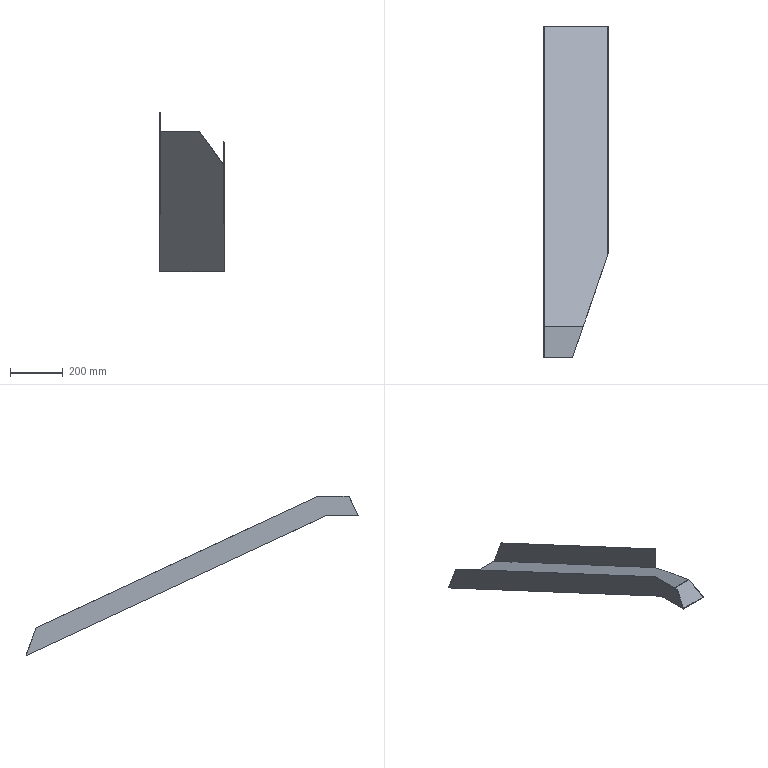Part | NX | features solid 2 | 1 solid | 14 faces | box 245 x 1262 x 605.091 mm | volume 969510 mm3 | plane 14
STEP:
#1=CARTESIAN_POINT('',(653.,254.738,-141.132));
#2=VERTEX_POINT('',#1);
#3=CARTESIAN_POINT('',(653.,1087.566,-529.486));
#4=VERTEX_POINT('',#3);
#5=CARTESIAN_POINT('',(653.,-205.417,73.442));
#6=DIRECTION('',(0.,-0.9063,0.4226));
#7=VECTOR('',#6,1000.);
#8=LINE('',#5,#7);
#9=EDGE_CURVE('',#2,#4,#8,.F.);
#10=ORIENTED_EDGE('',*,*,#9,.F.);
#11=CARTESIAN_POINT('',(655.,260.552,-143.843));
#12=VERTEX_POINT('',#11);
#13=CARTESIAN_POINT('',(451.78,-330.239,131.647));
#14=DIRECTION('',(0.2976,0.8652,-0.4035));
#15=VECTOR('',#14,1000.);
#16=LINE('',#13,#15);
#17=EDGE_CURVE('',#12,#2,#16,.F.);
#18=ORIENTED_EDGE('',*,*,#17,.F.);
#19=CARTESIAN_POINT('',(655.,1087.566,-529.486));
#20=VERTEX_POINT('',#19);
#21=CARTESIAN_POINT('',(655.,-205.417,73.442));
#22=DIRECTION('',(0.,-0.9063,0.4226));
#23=VECTOR('',#22,1000.);
#24=LINE('',#21,#23);
#25=EDGE_CURVE('',#12,#20,#24,.F.);
#26=ORIENTED_EDGE('',*,*,#25,.T.);
#27=CARTESIAN_POINT('',(10.,1087.566,-529.486));
#28=DIRECTION('',(1.,0.,0.));
#29=VECTOR('',#28,1000.);
#30=LINE('',#27,#29);
#31=EDGE_CURVE('',#4,#20,#30,.T.);
#32=ORIENTED_EDGE('',*,*,#31,.F.);
#33=EDGE_LOOP('',(#10,#18,#26,#32));
#34=FACE_BOUND('',#33,.T.);
#35=CARTESIAN_POINT('',(10.,-205.417,73.442));
#36=DIRECTION('',(0.,0.4226,0.9063));
#37=DIRECTION('',(0.,0.9063,-0.4226));
#38=AXIS2_PLACEMENT_3D('',#35,#36,#37);
#39=PLANE('',#38);
#40=ADVANCED_FACE('',(#34),#39,.T.);
#41=ORIENTED_EDGE('',*,*,#25,.F.);
#42=CARTESIAN_POINT('',(655.,260.552,-232.114));
#43=VERTEX_POINT('',#42);
#44=CARTESIAN_POINT('',(655.,260.552,73.442));
#45=DIRECTION('',(0.,0.,-1.));
#46=VECTOR('',#45,1000.);
#47=LINE('',#44,#46);
#48=EDGE_CURVE('',#12,#43,#47,.T.);
#49=ORIENTED_EDGE('',*,*,#48,.T.);
#50=CARTESIAN_POINT('',(655.,1126.262,-635.8));
#51=VERTEX_POINT('',#50);
#52=CARTESIAN_POINT('',(655.,-239.226,0.9369));
#53=DIRECTION('',(0.,-0.9063,0.4226));
#54=VECTOR('',#53,1000.);
#55=LINE('',#52,#54);
#56=EDGE_CURVE('',#43,#51,#55,.F.);
#57=ORIENTED_EDGE('',*,*,#56,.T.);
#58=CARTESIAN_POINT('',(655.,742.539,418.469));
#59=DIRECTION('',(0.,-0.342,0.9397));
#60=VECTOR('',#59,1000.);
#61=LINE('',#58,#60);
#62=EDGE_CURVE('',#20,#51,#61,.F.);
#63=ORIENTED_EDGE('',*,*,#62,.F.);
#64=EDGE_LOOP('',(#41,#49,#57,#63));
#65=FACE_BOUND('',#64,.T.);
#66=CARTESIAN_POINT('',(655.,-205.417,73.442));
#67=DIRECTION('',(1.,0.,0.));
#68=DIRECTION('',(0.,0.,1.));
#69=AXIS2_PLACEMENT_3D('',#66,#67,#68);
#70=PLANE('',#69);
#71=ADVANCED_FACE('',(#65),#70,.T.);
#72=CARTESIAN_POINT('',(410.,1126.262,-635.8));
#73=VERTEX_POINT('',#72);
#74=CARTESIAN_POINT('',(410.,-15.873,-103.215));
#75=VERTEX_POINT('',#74);
#76=CARTESIAN_POINT('',(410.,-239.226,0.9369));
#77=DIRECTION('',(0.,0.9063,-0.4226));
#78=VECTOR('',#77,1000.);
#79=LINE('',#76,#78);
#80=EDGE_CURVE('',#73,#75,#79,.F.);
#81=ORIENTED_EDGE('',*,*,#80,.T.);
#82=CARTESIAN_POINT('',(410.,-135.873,-103.215));
#83=VERTEX_POINT('',#82);
#84=CARTESIAN_POINT('',(410.,-135.873,-103.215));
#85=DIRECTION('',(0.,1.,0.));
#86=VECTOR('',#85,1000.);
#87=LINE('',#84,#86);
#88=EDGE_CURVE('',#83,#75,#87,.T.);
#89=ORIENTED_EDGE('',*,*,#88,.F.);
#90=CARTESIAN_POINT('',(410.,-102.063,-30.71));
#91=VERTEX_POINT('',#90);
#92=CARTESIAN_POINT('',(410.,-102.063,-30.71));
#93=DIRECTION('',(0.,-0.4226,-0.9063));
#94=VECTOR('',#93,1000.);
#95=LINE('',#92,#94);
#96=EDGE_CURVE('',#91,#83,#95,.T.);
#97=ORIENTED_EDGE('',*,*,#96,.F.);
#98=CARTESIAN_POINT('',(410.,17.937,-30.71));
#99=VERTEX_POINT('',#98);
#100=CARTESIAN_POINT('',(410.,-102.063,-30.71));
#101=DIRECTION('',(0.,1.,0.));
#102=VECTOR('',#101,1000.);
#103=LINE('',#100,#102);
#104=EDGE_CURVE('',#91,#99,#103,.T.);
#105=ORIENTED_EDGE('',*,*,#104,.T.);
#106=CARTESIAN_POINT('',(410.,1087.566,-529.486));
#107=VERTEX_POINT('',#106);
#108=CARTESIAN_POINT('',(410.,-205.417,73.442));
#109=DIRECTION('',(0.,0.9063,-0.4226));
#110=VECTOR('',#109,1000.);
#111=LINE('',#108,#110);
#112=EDGE_CURVE('',#107,#99,#111,.F.);
#113=ORIENTED_EDGE('',*,*,#112,.F.);
#114=CARTESIAN_POINT('',(410.,742.539,418.469));
#115=DIRECTION('',(0.,0.342,-0.9397));
#116=VECTOR('',#115,1000.);
#117=LINE('',#114,#116);
#118=EDGE_CURVE('',#73,#107,#117,.F.);
#119=ORIENTED_EDGE('',*,*,#118,.F.);
#120=EDGE_LOOP('',(#81,#89,#97,#105,#113,#119));
#121=FACE_BOUND('',#120,.T.);
#122=CARTESIAN_POINT('',(410.,-205.417,73.442));
#123=DIRECTION('',(-1.,0.,0.));
#124=DIRECTION('',(0.,0.,-1.));
#125=AXIS2_PLACEMENT_3D('',#122,#123,#124);
#126=PLANE('',#125);
#127=ADVANCED_FACE('',(#121),#126,.T.);
#128=ORIENTED_EDGE('',*,*,#112,.T.);
#129=CARTESIAN_POINT('',(412.,17.937,-30.71));
#130=VERTEX_POINT('',#129);
#131=CARTESIAN_POINT('',(10.,17.937,-30.71));
#132=DIRECTION('',(-1.,0.,0.));
#133=VECTOR('',#132,1000.);
#134=LINE('',#131,#133);
#135=EDGE_CURVE('',#99,#130,#134,.F.);
#136=ORIENTED_EDGE('',*,*,#135,.T.);
#137=CARTESIAN_POINT('',(412.,1087.566,-529.486));
#138=VERTEX_POINT('',#137);
#139=CARTESIAN_POINT('',(412.,-205.417,73.442));
#140=DIRECTION('',(0.,0.9063,-0.4226));
#141=VECTOR('',#140,1000.);
#142=LINE('',#139,#141);
#143=EDGE_CURVE('',#138,#130,#142,.F.);
#144=ORIENTED_EDGE('',*,*,#143,.F.);
#145=CARTESIAN_POINT('',(412.,1087.566,-529.486));
#146=DIRECTION('',(-1.,0.,0.));
#147=VECTOR('',#146,1000.);
#148=LINE('',#145,#147);
#149=EDGE_CURVE('',#107,#138,#148,.F.);
#150=ORIENTED_EDGE('',*,*,#149,.F.);
#151=EDGE_LOOP('',(#128,#136,#144,#150));
#152=FACE_BOUND('',#151,.T.);
#153=CARTESIAN_POINT('',(10.,-205.417,73.442));
#154=DIRECTION('',(0.,0.4226,0.9063));
#155=DIRECTION('',(0.,0.9063,-0.4226));
#156=AXIS2_PLACEMENT_3D('',#153,#154,#155);
#157=PLANE('',#156);
#158=ADVANCED_FACE('',(#152),#157,.T.);
#159=CARTESIAN_POINT('',(559.915,-15.873,-103.215));
#160=VERTEX_POINT('',#159);
#161=CARTESIAN_POINT('',(441.18,-361.053,57.746));
#162=DIRECTION('',(0.2976,0.8652,-0.4035));
#163=VECTOR('',#162,1000.);
#164=LINE('',#161,#163);
#165=EDGE_CURVE('',#43,#160,#164,.F.);
#166=ORIENTED_EDGE('',*,*,#165,.T.);
#167=CARTESIAN_POINT('',(10.,-15.873,-103.215));
#168=DIRECTION('',(-1.,0.,0.));
#169=VECTOR('',#168,1000.);
#170=LINE('',#167,#169);
#171=EDGE_CURVE('',#75,#160,#170,.F.);
#172=ORIENTED_EDGE('',*,*,#171,.F.);
#173=ORIENTED_EDGE('',*,*,#80,.F.);
#174=CARTESIAN_POINT('',(10.,1126.262,-635.8));
#175=DIRECTION('',(1.,0.,0.));
#176=VECTOR('',#175,1000.);
#177=LINE('',#174,#176);
#178=EDGE_CURVE('',#51,#73,#177,.F.);
#179=ORIENTED_EDGE('',*,*,#178,.F.);
#180=ORIENTED_EDGE('',*,*,#56,.F.);
#181=EDGE_LOOP('',(#166,#172,#173,#179,#180));
#182=FACE_BOUND('',#181,.T.);
#183=CARTESIAN_POINT('',(10.,-239.226,0.9369));
#184=DIRECTION('',(0.,0.4226,0.9063));
#185=DIRECTION('',(0.,0.9063,-0.4226));
#186=AXIS2_PLACEMENT_3D('',#183,#184,#185);
#187=PLANE('',#186);
#188=ADVANCED_FACE('',(#182),#187,.F.);
#189=CARTESIAN_POINT('',(653.,254.738,-227.196));
#190=VERTEX_POINT('',#189);
#191=CARTESIAN_POINT('',(653.,1125.294,-633.143));
#192=VERTEX_POINT('',#191);
#193=CARTESIAN_POINT('',(653.,-238.381,2.75));
#194=DIRECTION('',(0.,-0.9063,0.4226));
#195=VECTOR('',#194,1000.);
#196=LINE('',#193,#195);
#197=EDGE_CURVE('',#190,#192,#196,.F.);
#198=ORIENTED_EDGE('',*,*,#197,.F.);
#199=CARTESIAN_POINT('',(653.,254.738,73.442));
#200=DIRECTION('',(0.,0.,-1.));
#201=VECTOR('',#200,1000.);
#202=LINE('',#199,#201);
#203=EDGE_CURVE('',#2,#190,#202,.T.);
#204=ORIENTED_EDGE('',*,*,#203,.F.);
#205=ORIENTED_EDGE('',*,*,#9,.T.);
#206=CARTESIAN_POINT('',(653.,1126.262,-635.8));
#207=DIRECTION('',(0.,0.342,-0.9397));
#208=VECTOR('',#207,1000.);
#209=LINE('',#206,#208);
#210=EDGE_CURVE('',#192,#4,#209,.F.);
#211=ORIENTED_EDGE('',*,*,#210,.F.);
#212=EDGE_LOOP('',(#198,#204,#205,#211));
#213=FACE_BOUND('',#212,.T.);
#214=CARTESIAN_POINT('',(653.,-205.417,73.442));
#215=DIRECTION('',(1.,0.,0.));
#216=DIRECTION('',(0.,0.,1.));
#217=AXIS2_PLACEMENT_3D('',#214,#215,#216);
#218=PLANE('',#217);
#219=ADVANCED_FACE('',(#213),#218,.F.);
#220=ORIENTED_EDGE('',*,*,#143,.T.);
#221=CARTESIAN_POINT('',(412.,-102.063,-30.71));
#222=VERTEX_POINT('',#221);
#223=CARTESIAN_POINT('',(412.,-102.063,-30.71));
#224=DIRECTION('',(0.,1.,0.));
#225=VECTOR('',#224,1000.);
#226=LINE('',#223,#225);
#227=EDGE_CURVE('',#222,#130,#226,.T.);
#228=ORIENTED_EDGE('',*,*,#227,.F.);
#229=CARTESIAN_POINT('',(412.,-135.027,-101.402));
#230=VERTEX_POINT('',#229);
#231=CARTESIAN_POINT('',(412.,-102.063,-30.71));
#232=DIRECTION('',(0.,-0.4226,-0.9063));
#233=VECTOR('',#232,1000.);
#234=LINE('',#231,#233);
#235=EDGE_CURVE('',#222,#230,#234,.T.);
#236=ORIENTED_EDGE('',*,*,#235,.T.);
#237=CARTESIAN_POINT('',(412.,-15.027,-101.402));
#238=VERTEX_POINT('',#237);
#239=CARTESIAN_POINT('',(412.,-135.027,-101.402));
#240=DIRECTION('',(0.,1.,0.));
#241=VECTOR('',#240,1000.);
#242=LINE('',#239,#241);
#243=EDGE_CURVE('',#230,#238,#242,.T.);
#244=ORIENTED_EDGE('',*,*,#243,.T.);
#245=CARTESIAN_POINT('',(412.,1125.294,-633.143));
#246=VERTEX_POINT('',#245);
#247=CARTESIAN_POINT('',(412.,-238.381,2.75));
#248=DIRECTION('',(0.,0.9063,-0.4226));
#249=VECTOR('',#248,1000.);
#250=LINE('',#247,#249);
#251=EDGE_CURVE('',#246,#238,#250,.F.);
#252=ORIENTED_EDGE('',*,*,#251,.F.);
#253=CARTESIAN_POINT('',(412.,1126.262,-635.8));
#254=DIRECTION('',(0.,-0.342,0.9397));
#255=VECTOR('',#254,1000.);
#256=LINE('',#253,#255);
#257=EDGE_CURVE('',#138,#246,#256,.F.);
#258=ORIENTED_EDGE('',*,*,#257,.F.);
#259=EDGE_LOOP('',(#220,#228,#236,#244,#252,#258));
#260=FACE_BOUND('',#259,.T.);
#261=CARTESIAN_POINT('',(412.,-205.417,73.442));
#262=DIRECTION('',(-1.,0.,0.));
#263=DIRECTION('',(0.,0.,-1.));
#264=AXIS2_PLACEMENT_3D('',#261,#262,#263);
#265=PLANE('',#264);
#266=ADVANCED_FACE('',(#260),#265,.F.);
#267=ORIENTED_EDGE('',*,*,#251,.T.);
#268=CARTESIAN_POINT('',(560.206,-15.027,-101.402));
#269=VERTEX_POINT('',#268);
#270=CARTESIAN_POINT('',(10.,-15.027,-101.402));
#271=DIRECTION('',(-1.,0.,0.));
#272=VECTOR('',#271,1000.);
#273=LINE('',#270,#272);
#274=EDGE_CURVE('',#238,#269,#273,.F.);
#275=ORIENTED_EDGE('',*,*,#274,.T.);
#276=CARTESIAN_POINT('',(441.445,-360.283,59.593));
#277=DIRECTION('',(0.2976,0.8652,-0.4035));
#278=VECTOR('',#277,1000.);
#279=LINE('',#276,#278);
#280=EDGE_CURVE('',#190,#269,#279,.F.);
#281=ORIENTED_EDGE('',*,*,#280,.F.);
#282=ORIENTED_EDGE('',*,*,#197,.T.);
#283=CARTESIAN_POINT('',(10.,1125.294,-633.143));
#284=DIRECTION('',(1.,0.,0.));
#285=VECTOR('',#284,1000.);
#286=LINE('',#283,#285);
#287=EDGE_CURVE('',#246,#192,#286,.T.);
#288=ORIENTED_EDGE('',*,*,#287,.F.);
#289=EDGE_LOOP('',(#267,#275,#281,#282,#288));
#290=FACE_BOUND('',#289,.T.);
#291=CARTESIAN_POINT('',(10.,-238.381,2.75));
#292=DIRECTION('',(0.,0.4226,0.9063));
#293=DIRECTION('',(0.,0.9063,-0.4226));
#294=AXIS2_PLACEMENT_3D('',#291,#292,#293);
#295=PLANE('',#294);
#296=ADVANCED_FACE('',(#290),#295,.T.);
#297=ORIENTED_EDGE('',*,*,#135,.F.);
#298=ORIENTED_EDGE('',*,*,#104,.F.);
#299=CARTESIAN_POINT('',(10.,-102.063,-30.71));
#300=DIRECTION('',(-1.,0.,0.));
#301=VECTOR('',#300,1000.);
#302=LINE('',#299,#301);
#303=EDGE_CURVE('',#91,#222,#302,.F.);
#304=ORIENTED_EDGE('',*,*,#303,.T.);
#305=ORIENTED_EDGE('',*,*,#227,.T.);
#306=EDGE_LOOP('',(#297,#298,#304,#305));
#307=FACE_BOUND('',#306,.T.);
#308=CARTESIAN_POINT('',(10.,-102.063,-30.71));
#309=DIRECTION('',(0.,0.,-1.));
#310=DIRECTION('',(1.,0.,0.));
#311=AXIS2_PLACEMENT_3D('',#308,#309,#310);
#312=PLANE('',#311);
#313=ADVANCED_FACE('',(#307),#312,.F.);
#314=ORIENTED_EDGE('',*,*,#274,.F.);
#315=ORIENTED_EDGE('',*,*,#243,.F.);
#316=CARTESIAN_POINT('',(518.928,-135.027,-101.402));
#317=VERTEX_POINT('',#316);
#318=CARTESIAN_POINT('',(10.,-135.027,-101.402));
#319=DIRECTION('',(-1.,0.,0.));
#320=VECTOR('',#319,1000.);
#321=LINE('',#318,#320);
#322=EDGE_CURVE('',#230,#317,#321,.F.);
#323=ORIENTED_EDGE('',*,*,#322,.T.);
#324=CARTESIAN_POINT('',(465.082,-291.567,-101.402));
#325=DIRECTION('',(-0.3253,-0.9456,0.));
#326=VECTOR('',#325,1000.);
#327=LINE('',#324,#326);
#328=EDGE_CURVE('',#269,#317,#327,.T.);
#329=ORIENTED_EDGE('',*,*,#328,.F.);
#330=EDGE_LOOP('',(#314,#315,#323,#329));
#331=FACE_BOUND('',#330,.T.);
#332=CARTESIAN_POINT('',(10.,-135.027,-101.402));
#333=DIRECTION('',(0.,0.,-1.));
#334=DIRECTION('',(1.,0.,0.));
#335=AXIS2_PLACEMENT_3D('',#332,#333,#334);
#336=PLANE('',#335);
#337=ADVANCED_FACE('',(#331),#336,.F.);
#338=CARTESIAN_POINT('',(518.638,-135.873,-103.215));
#339=VERTEX_POINT('',#338);
#340=CARTESIAN_POINT('',(464.822,-292.323,-103.215));
#341=DIRECTION('',(-0.3253,-0.9456,0.));
#342=VECTOR('',#341,1000.);
#343=LINE('',#340,#342);
#344=EDGE_CURVE('',#160,#339,#343,.T.);
#345=ORIENTED_EDGE('',*,*,#344,.T.);
#346=CARTESIAN_POINT('',(10.,-135.873,-103.215));
#347=DIRECTION('',(-1.,0.,0.));
#348=VECTOR('',#347,1000.);
#349=LINE('',#346,#348);
#350=EDGE_CURVE('',#83,#339,#349,.F.);
#351=ORIENTED_EDGE('',*,*,#350,.F.);
#352=ORIENTED_EDGE('',*,*,#88,.T.);
#353=ORIENTED_EDGE('',*,*,#171,.T.);
#354=EDGE_LOOP('',(#345,#351,#352,#353));
#355=FACE_BOUND('',#354,.T.);
#356=CARTESIAN_POINT('',(10.,-135.873,-103.215));
#357=DIRECTION('',(0.,0.,-1.));
#358=DIRECTION('',(1.,0.,0.));
#359=AXIS2_PLACEMENT_3D('',#356,#357,#358);
#360=PLANE('',#359);
#361=ADVANCED_FACE('',(#355),#360,.T.);
#362=CARTESIAN_POINT('',(544.335,-61.167,56.993));
#363=DIRECTION('',(0.1439,0.4182,0.8969));
#364=VECTOR('',#363,1000.);
#365=LINE('',#362,#364);
#366=EDGE_CURVE('',#339,#317,#365,.T.);
#367=ORIENTED_EDGE('',*,*,#366,.T.);
#368=ORIENTED_EDGE('',*,*,#322,.F.);
#369=ORIENTED_EDGE('',*,*,#235,.F.);
#370=ORIENTED_EDGE('',*,*,#303,.F.);
#371=ORIENTED_EDGE('',*,*,#96,.T.);
#372=ORIENTED_EDGE('',*,*,#350,.T.);
#373=EDGE_LOOP('',(#367,#368,#369,#370,#371,#372));
#374=FACE_BOUND('',#373,.T.);
#375=CARTESIAN_POINT('',(1210.,-102.063,-30.71));
#376=DIRECTION('',(0.,-0.9063,0.4226));
#377=DIRECTION('',(0.,-0.4226,-0.9063));
#378=AXIS2_PLACEMENT_3D('',#375,#376,#377);
#379=PLANE('',#378);
#380=ADVANCED_FACE('',(#374),#379,.T.);
#381=ORIENTED_EDGE('',*,*,#17,.T.);
#382=ORIENTED_EDGE('',*,*,#203,.T.);
#383=ORIENTED_EDGE('',*,*,#280,.T.);
#384=ORIENTED_EDGE('',*,*,#328,.T.);
#385=ORIENTED_EDGE('',*,*,#366,.F.);
#386=ORIENTED_EDGE('',*,*,#344,.F.);
#387=ORIENTED_EDGE('',*,*,#165,.F.);
#388=ORIENTED_EDGE('',*,*,#48,.F.);
#389=EDGE_LOOP('',(#381,#382,#383,#384,#385,#386,#387,#388));
#390=FACE_BOUND('',#389,.T.);
#391=CARTESIAN_POINT('',(518.565,-136.085,0.));
#392=DIRECTION('',(-0.9456,0.3253,0.));
#393=DIRECTION('',(0.3253,0.9456,0.));
#394=AXIS2_PLACEMENT_3D('',#391,#392,#393);
#395=PLANE('',#394);
#396=ADVANCED_FACE('',(#390),#395,.F.);
#397=ORIENTED_EDGE('',*,*,#257,.T.);
#398=ORIENTED_EDGE('',*,*,#287,.T.);
#399=ORIENTED_EDGE('',*,*,#210,.T.);
#400=ORIENTED_EDGE('',*,*,#31,.T.);
#401=ORIENTED_EDGE('',*,*,#62,.T.);
#402=ORIENTED_EDGE('',*,*,#178,.T.);
#403=ORIENTED_EDGE('',*,*,#118,.T.);
#404=ORIENTED_EDGE('',*,*,#149,.T.);
#405=EDGE_LOOP('',(#397,#398,#399,#400,#401,#402,#403,#404));
#406=FACE_BOUND('',#405,.T.);
#407=CARTESIAN_POINT('',(10.,1126.262,-635.8));
#408=DIRECTION('',(0.,-0.9397,-0.342));
#409=DIRECTION('',(0.,0.342,-0.9397));
#410=AXIS2_PLACEMENT_3D('',#407,#408,#409);
#411=PLANE('',#410);
#412=ADVANCED_FACE('',(#406),#411,.F.);
#413=CLOSED_SHELL('',(#40,#71,#127,#158,#188,#219,#266,#296,#313,#337,#361,#380,#396,#412));
#414=MANIFOLD_SOLID_BREP('',#413);
#415=(LENGTH_UNIT()NAMED_UNIT(*)SI_UNIT(.MILLI.,.METRE.));
#416=UNCERTAINTY_MEASURE_WITH_UNIT(LENGTH_MEASURE(0.00001),#415,'','');
#417=(NAMED_UNIT(*)PLANE_ANGLE_UNIT()SI_UNIT($,.RADIAN.));
#418=(NAMED_UNIT(*)SI_UNIT($,.STERADIAN.)SOLID_ANGLE_UNIT());
#419=(GEOMETRIC_REPRESENTATION_CONTEXT(3)GLOBAL_UNCERTAINTY_ASSIGNED_CONTEXT((#416))GLOBAL_UNIT_ASSIGNED_CONTEXT((#415,#417,#418))REPRESENTATION_CONTEXT('',''));
#420=ADVANCED_BREP_SHAPE_REPRESENTATION('',(#414),#419);